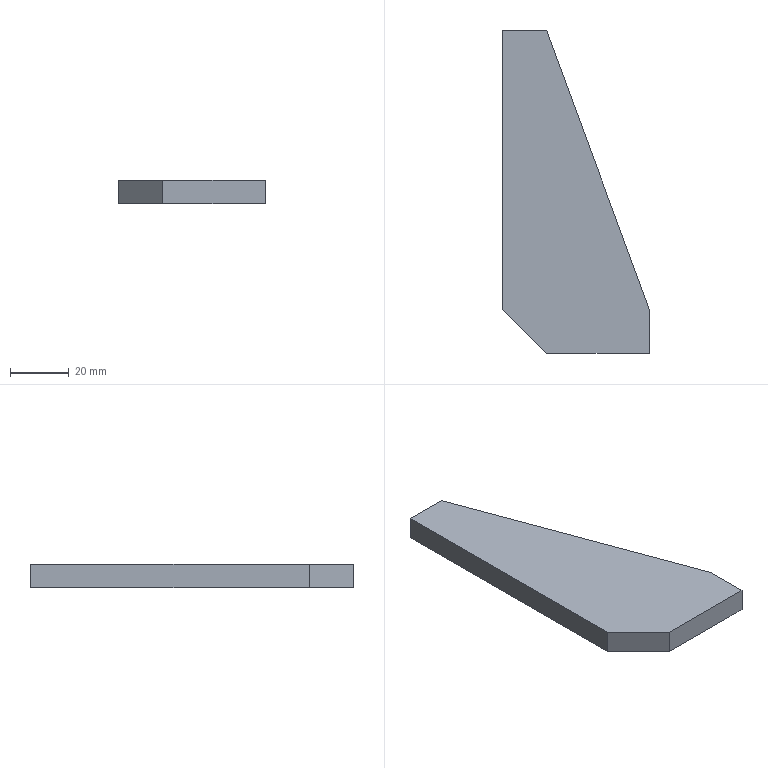Part | SolidWorks | features Chamfer 1, Extrusion 1 | 1 solid | 8 faces | box 50 x 110 x 8 mm | volume 29800 mm3 | plane 8
STEP:
#1=CARTESIAN_POINT('',(0.,110.,0.));
#2=VERTEX_POINT('',#1);
#3=CARTESIAN_POINT('',(0.,15.,0.));
#4=VERTEX_POINT('',#3);
#5=CARTESIAN_POINT('',(0.,110.,0.));
#6=DIRECTION('',(0.,-1.,0.));
#7=VECTOR('',#6,1000.);
#8=LINE('',#5,#7);
#9=EDGE_CURVE('',#2,#4,#8,.T.);
#10=ORIENTED_EDGE('',*,*,#9,.T.);
#11=CARTESIAN_POINT('',(0.,15.,8.));
#12=VERTEX_POINT('',#11);
#13=CARTESIAN_POINT('',(0.,15.,8.));
#14=DIRECTION('',(0.,0.,1.));
#15=VECTOR('',#14,1000.);
#16=LINE('',#13,#15);
#17=EDGE_CURVE('',#4,#12,#16,.T.);
#18=ORIENTED_EDGE('',*,*,#17,.T.);
#19=CARTESIAN_POINT('',(0.,110.,8.));
#20=VERTEX_POINT('',#19);
#21=CARTESIAN_POINT('',(0.,110.,8.));
#22=DIRECTION('',(0.,-1.,0.));
#23=VECTOR('',#22,1000.);
#24=LINE('',#21,#23);
#25=EDGE_CURVE('',#20,#12,#24,.T.);
#26=ORIENTED_EDGE('',*,*,#25,.F.);
#27=CARTESIAN_POINT('',(0.,110.,8.));
#28=DIRECTION('',(0.,0.,-1.));
#29=VECTOR('',#28,1000.);
#30=LINE('',#27,#29);
#31=EDGE_CURVE('',#20,#2,#30,.T.);
#32=ORIENTED_EDGE('',*,*,#31,.T.);
#33=EDGE_LOOP('',(#10,#18,#26,#32));
#34=FACE_OUTER_BOUND('',#33,.T.);
#35=CARTESIAN_POINT('',(0.,110.,8.));
#36=DIRECTION('',(1.,0.,0.));
#37=DIRECTION('',(0.,1.,0.));
#38=AXIS2_PLACEMENT_3D('',#35,#36,#37);
#39=PLANE('',#38);
#40=ADVANCED_FACE('',(#34),#39,.F.);
#41=CARTESIAN_POINT('',(15.,0.,8.));
#42=VERTEX_POINT('',#41);
#43=CARTESIAN_POINT('',(50.,0.,8.));
#44=VERTEX_POINT('',#43);
#45=CARTESIAN_POINT('',(0.,0.,8.));
#46=DIRECTION('',(1.,0.,0.));
#47=VECTOR('',#46,1000.);
#48=LINE('',#45,#47);
#49=EDGE_CURVE('',#42,#44,#48,.T.);
#50=ORIENTED_EDGE('',*,*,#49,.F.);
#51=CARTESIAN_POINT('',(15.,0.,0.));
#52=VERTEX_POINT('',#51);
#53=CARTESIAN_POINT('',(15.,0.,8.));
#54=DIRECTION('',(0.,0.,-1.));
#55=VECTOR('',#54,1000.);
#56=LINE('',#53,#55);
#57=EDGE_CURVE('',#42,#52,#56,.T.);
#58=ORIENTED_EDGE('',*,*,#57,.T.);
#59=CARTESIAN_POINT('',(50.,0.,0.));
#60=VERTEX_POINT('',#59);
#61=CARTESIAN_POINT('',(0.,0.,0.));
#62=DIRECTION('',(1.,0.,0.));
#63=VECTOR('',#62,1000.);
#64=LINE('',#61,#63);
#65=EDGE_CURVE('',#52,#60,#64,.T.);
#66=ORIENTED_EDGE('',*,*,#65,.T.);
#67=CARTESIAN_POINT('',(50.,0.,8.));
#68=DIRECTION('',(0.,0.,-1.));
#69=VECTOR('',#68,1000.);
#70=LINE('',#67,#69);
#71=EDGE_CURVE('',#44,#60,#70,.T.);
#72=ORIENTED_EDGE('',*,*,#71,.F.);
#73=EDGE_LOOP('',(#50,#58,#66,#72));
#74=FACE_OUTER_BOUND('',#73,.T.);
#75=CARTESIAN_POINT('',(0.,0.,8.));
#76=DIRECTION('',(0.,1.,0.));
#77=DIRECTION('',(0.,0.,1.));
#78=AXIS2_PLACEMENT_3D('',#75,#76,#77);
#79=PLANE('',#78);
#80=ADVANCED_FACE('',(#74),#79,.F.);
#81=CARTESIAN_POINT('',(50.,15.,0.));
#82=VERTEX_POINT('',#81);
#83=CARTESIAN_POINT('',(50.,0.,0.));
#84=DIRECTION('',(0.,1.,0.));
#85=VECTOR('',#84,1000.);
#86=LINE('',#83,#85);
#87=EDGE_CURVE('',#60,#82,#86,.T.);
#88=ORIENTED_EDGE('',*,*,#87,.T.);
#89=CARTESIAN_POINT('',(50.,15.,8.));
#90=VERTEX_POINT('',#89);
#91=CARTESIAN_POINT('',(50.,15.,8.));
#92=DIRECTION('',(0.,0.,-1.));
#93=VECTOR('',#92,1000.);
#94=LINE('',#91,#93);
#95=EDGE_CURVE('',#90,#82,#94,.T.);
#96=ORIENTED_EDGE('',*,*,#95,.F.);
#97=CARTESIAN_POINT('',(50.,0.,8.));
#98=DIRECTION('',(0.,1.,0.));
#99=VECTOR('',#98,1000.);
#100=LINE('',#97,#99);
#101=EDGE_CURVE('',#44,#90,#100,.T.);
#102=ORIENTED_EDGE('',*,*,#101,.F.);
#103=ORIENTED_EDGE('',*,*,#71,.T.);
#104=EDGE_LOOP('',(#88,#96,#102,#103));
#105=FACE_OUTER_BOUND('',#104,.T.);
#106=CARTESIAN_POINT('',(50.,0.,8.));
#107=DIRECTION('',(-1.,0.,0.));
#108=DIRECTION('',(0.,0.,1.));
#109=AXIS2_PLACEMENT_3D('',#106,#107,#108);
#110=PLANE('',#109);
#111=ADVANCED_FACE('',(#105),#110,.F.);
#112=CARTESIAN_POINT('',(15.,110.,0.));
#113=VERTEX_POINT('',#112);
#114=CARTESIAN_POINT('',(50.,15.,0.));
#115=DIRECTION('',(-0.3457,0.9383,0.));
#116=VECTOR('',#115,1000.);
#117=LINE('',#114,#116);
#118=EDGE_CURVE('',#82,#113,#117,.T.);
#119=ORIENTED_EDGE('',*,*,#118,.T.);
#120=CARTESIAN_POINT('',(15.,110.,8.));
#121=VERTEX_POINT('',#120);
#122=CARTESIAN_POINT('',(15.,110.,8.));
#123=DIRECTION('',(0.,0.,-1.));
#124=VECTOR('',#123,1000.);
#125=LINE('',#122,#124);
#126=EDGE_CURVE('',#121,#113,#125,.T.);
#127=ORIENTED_EDGE('',*,*,#126,.F.);
#128=CARTESIAN_POINT('',(50.,15.,8.));
#129=DIRECTION('',(-0.3457,0.9383,0.));
#130=VECTOR('',#129,1000.);
#131=LINE('',#128,#130);
#132=EDGE_CURVE('',#90,#121,#131,.T.);
#133=ORIENTED_EDGE('',*,*,#132,.F.);
#134=ORIENTED_EDGE('',*,*,#95,.T.);
#135=EDGE_LOOP('',(#119,#127,#133,#134));
#136=FACE_OUTER_BOUND('',#135,.T.);
#137=CARTESIAN_POINT('',(50.,15.,8.));
#138=DIRECTION('',(-0.9383,-0.3457,0.));
#139=DIRECTION('',(0.3457,-0.9383,0.));
#140=AXIS2_PLACEMENT_3D('',#137,#138,#139);
#141=PLANE('',#140);
#142=ADVANCED_FACE('',(#136),#141,.F.);
#143=CARTESIAN_POINT('',(15.,110.,0.));
#144=DIRECTION('',(-1.,0.,0.));
#145=VECTOR('',#144,1000.);
#146=LINE('',#143,#145);
#147=EDGE_CURVE('',#113,#2,#146,.T.);
#148=ORIENTED_EDGE('',*,*,#147,.T.);
#149=ORIENTED_EDGE('',*,*,#31,.F.);
#150=CARTESIAN_POINT('',(15.,110.,8.));
#151=DIRECTION('',(-1.,0.,0.));
#152=VECTOR('',#151,1000.);
#153=LINE('',#150,#152);
#154=EDGE_CURVE('',#121,#20,#153,.T.);
#155=ORIENTED_EDGE('',*,*,#154,.F.);
#156=ORIENTED_EDGE('',*,*,#126,.T.);
#157=EDGE_LOOP('',(#148,#149,#155,#156));
#158=FACE_OUTER_BOUND('',#157,.T.);
#159=CARTESIAN_POINT('',(15.,110.,8.));
#160=DIRECTION('',(0.,-1.,0.));
#161=DIRECTION('',(0.,0.,-1.));
#162=AXIS2_PLACEMENT_3D('',#159,#160,#161);
#163=PLANE('',#162);
#164=ADVANCED_FACE('',(#158),#163,.F.);
#165=ORIENTED_EDGE('',*,*,#25,.T.);
#166=CARTESIAN_POINT('',(7.5,7.5,8.));
#167=DIRECTION('',(0.7071,-0.7071,0.));
#168=VECTOR('',#167,1000.);
#169=LINE('',#166,#168);
#170=EDGE_CURVE('',#12,#42,#169,.T.);
#171=ORIENTED_EDGE('',*,*,#170,.T.);
#172=ORIENTED_EDGE('',*,*,#49,.T.);
#173=ORIENTED_EDGE('',*,*,#101,.T.);
#174=ORIENTED_EDGE('',*,*,#132,.T.);
#175=ORIENTED_EDGE('',*,*,#154,.T.);
#176=EDGE_LOOP('',(#165,#171,#172,#173,#174,#175));
#177=FACE_OUTER_BOUND('',#176,.T.);
#178=CARTESIAN_POINT('',(0.,0.,8.));
#179=DIRECTION('',(0.,0.,1.));
#180=DIRECTION('',(1.,0.,0.));
#181=AXIS2_PLACEMENT_3D('',#178,#179,#180);
#182=PLANE('',#181);
#183=ADVANCED_FACE('',(#177),#182,.T.);
#184=ORIENTED_EDGE('',*,*,#65,.F.);
#185=CARTESIAN_POINT('',(15.,0.,0.));
#186=DIRECTION('',(-0.7071,0.7071,0.));
#187=VECTOR('',#186,1000.);
#188=LINE('',#185,#187);
#189=EDGE_CURVE('',#52,#4,#188,.T.);
#190=ORIENTED_EDGE('',*,*,#189,.T.);
#191=ORIENTED_EDGE('',*,*,#9,.F.);
#192=ORIENTED_EDGE('',*,*,#147,.F.);
#193=ORIENTED_EDGE('',*,*,#118,.F.);
#194=ORIENTED_EDGE('',*,*,#87,.F.);
#195=EDGE_LOOP('',(#184,#190,#191,#192,#193,#194));
#196=FACE_OUTER_BOUND('',#195,.T.);
#197=CARTESIAN_POINT('',(0.,0.,0.));
#198=DIRECTION('',(0.,0.,1.));
#199=DIRECTION('',(1.,0.,0.));
#200=AXIS2_PLACEMENT_3D('',#197,#198,#199);
#201=PLANE('',#200);
#202=ADVANCED_FACE('',(#196),#201,.F.);
#203=ORIENTED_EDGE('',*,*,#170,.F.);
#204=ORIENTED_EDGE('',*,*,#17,.F.);
#205=ORIENTED_EDGE('',*,*,#189,.F.);
#206=ORIENTED_EDGE('',*,*,#57,.F.);
#207=EDGE_LOOP('',(#203,#204,#205,#206));
#208=FACE_OUTER_BOUND('',#207,.T.);
#209=CARTESIAN_POINT('',(15.,0.,8.));
#210=DIRECTION('',(0.7071,0.7071,0.));
#211=DIRECTION('',(0.,0.,-1.));
#212=AXIS2_PLACEMENT_3D('',#209,#210,#211);
#213=PLANE('',#212);
#214=ADVANCED_FACE('',(#208),#213,.F.);
#215=CLOSED_SHELL('',(#40,#80,#111,#142,#164,#183,#202,#214));
#216=MANIFOLD_SOLID_BREP('',#215);
#217=CARTESIAN_POINT('',(0.,0.,0.));
#218=DIRECTION('',(0.,0.,1.));
#219=DIRECTION('',(1.,0.,0.));
#220=AXIS2_PLACEMENT_3D('',#217,#218,#219);
#221=(LENGTH_UNIT()NAMED_UNIT(*)SI_UNIT(.MILLI.,.METRE.));
#222=UNCERTAINTY_MEASURE_WITH_UNIT(LENGTH_MEASURE(0.00001),#221,'','');
#223=(NAMED_UNIT(*)PLANE_ANGLE_UNIT()SI_UNIT($,.RADIAN.));
#224=(NAMED_UNIT(*)SI_UNIT($,.STERADIAN.)SOLID_ANGLE_UNIT());
#225=(GEOMETRIC_REPRESENTATION_CONTEXT(3)GLOBAL_UNCERTAINTY_ASSIGNED_CONTEXT((#222))GLOBAL_UNIT_ASSIGNED_CONTEXT((#221,#223,#224))REPRESENTATION_CONTEXT('',''));
#226=ADVANCED_BREP_SHAPE_REPRESENTATION('',(#216,#220),#225);